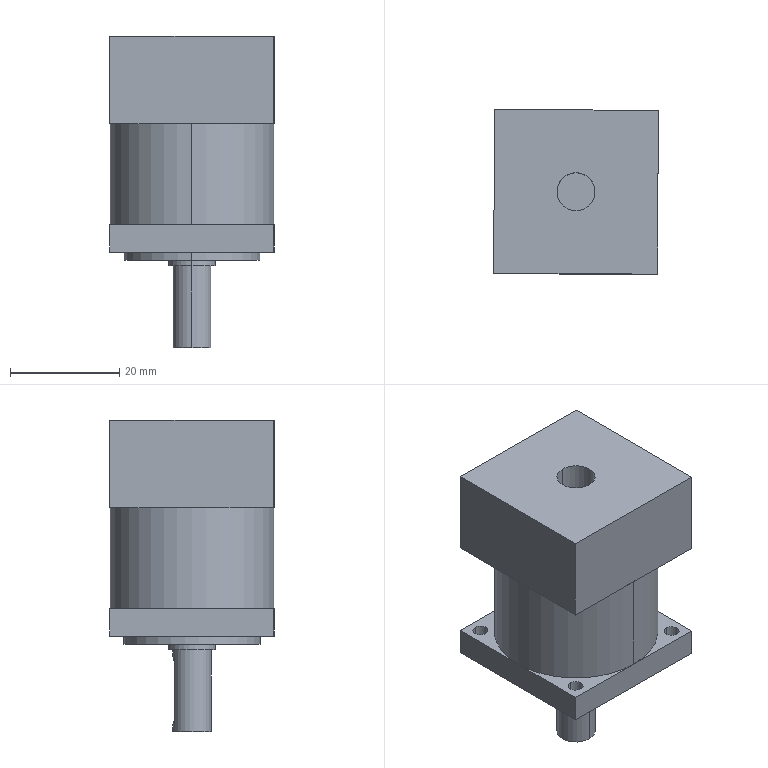Part | STEP file | 2026.6.15-Main Assembly图.sldasm-Part-157 | 1 solid | 47 faces | box 30.153 x 30.153 x 57 mm | volume 32608 mm3 | plane 25 | cylinder 22 | commonest cylinder face diameters 2.75 x8 2.5 x4 7 x4 8.5 x2 25 x2 30 x2
STEP:
#1=CARTESIAN_POINT('',(-1556.397,1436.505,3721.32));
#2=VERTEX_POINT('',#1);
#3=CARTESIAN_POINT('',(-1555.189,1436.504,3720.071));
#4=VERTEX_POINT('',#3);
#5=CARTESIAN_POINT('',(-1556.439,1436.505,3720.071));
#6=DIRECTION('',(0.0007664,1.,0.));
#7=DIRECTION('',(0.03353,-0.0000257,0.9994));
#8=AXIS2_PLACEMENT_3D('',#5,#6,#7);
#9=CIRCLE('',#8,1.25);
#10=EDGE_CURVE('',#2,#4,#9,.T.);
#11=ORIENTED_EDGE('',*,*,#10,.F.);
#12=CARTESIAN_POINT('',(-1556.396,1438.004,3721.32));
#13=VERTEX_POINT('',#12);
#14=CARTESIAN_POINT('',(-1556.395,1439.005,3721.32));
#15=DIRECTION('',(0.0007664,1.,0.));
#16=VECTOR('',#15,1000.);
#17=LINE('',#14,#16);
#18=EDGE_CURVE('',#2,#13,#17,.T.);
#19=ORIENTED_EDGE('',*,*,#18,.T.);
#20=CARTESIAN_POINT('',(-1555.188,1437.767,3720.071));
#21=VERTEX_POINT('',#20);
#22=CARTESIAN_POINT('',(-1555.188,1437.767,3720.071));
#23=CARTESIAN_POINT('',(-1555.188,1437.767,3720.234));
#24=CARTESIAN_POINT('',(-1555.22,1437.78,3720.394));
#25=CARTESIAN_POINT('',(-1555.341,1437.823,3720.691));
#26=CARTESIAN_POINT('',(-1555.43,1437.853,3720.826));
#27=CARTESIAN_POINT('',(-1555.65,1437.913,3721.054));
#28=CARTESIAN_POINT('',(-1555.783,1437.943,3721.147));
#29=CARTESIAN_POINT('',(-1556.073,1437.987,3721.277));
#30=CARTESIAN_POINT('',(-1556.234,1438.002,3721.315));
#31=CARTESIAN_POINT('',(-1556.396,1438.004,3721.32));
#32=B_SPLINE_CURVE_WITH_KNOTS('',3,(#22,#23,#24,#25,#26,#27,#28,#29,#30,#31),.UNSPECIFIED.,.F.,.F.,(4,2,2,2,4),(0.,0.0004821,0.0009642,0.001446,0.001928),.UNSPECIFIED.);
#33=EDGE_CURVE('',#21,#13,#32,.T.);
#34=ORIENTED_EDGE('',*,*,#33,.F.);
#35=CARTESIAN_POINT('',(-1555.187,1439.004,3720.071));
#36=DIRECTION('',(0.0007664,1.,0.));
#37=VECTOR('',#36,1000.);
#38=LINE('',#35,#37);
#39=EDGE_CURVE('',#4,#21,#38,.T.);
#40=ORIENTED_EDGE('',*,*,#39,.F.);
#41=EDGE_LOOP('',(#11,#19,#34,#40));
#42=FACE_OUTER_BOUND('',#41,.T.);
#43=CARTESIAN_POINT('',(-1556.437,1439.005,3720.071));
#44=DIRECTION('',(0.0007664,1.,0.));
#45=DIRECTION('',(0.03353,-0.0000257,0.9994));
#46=AXIS2_PLACEMENT_3D('',#43,#44,#45);
#47=CYLINDRICAL_SURFACE('',#46,1.25);
#48=ADVANCED_FACE('',(#42),#47,.F.);
#49=CARTESIAN_POINT('',(-1556.48,1438.005,3708.821));
#50=VERTEX_POINT('',#49);
#51=CARTESIAN_POINT('',(-1556.453,1438.005,3708.821));
#52=VERTEX_POINT('',#51);
#53=CARTESIAN_POINT('',(-1556.48,1438.005,3708.821));
#54=CARTESIAN_POINT('',(-1556.471,1438.005,3708.821));
#55=CARTESIAN_POINT('',(-1556.462,1438.005,3708.821));
#56=CARTESIAN_POINT('',(-1556.453,1438.005,3708.821));
#57=B_SPLINE_CURVE_WITH_KNOTS('',3,(#53,#54,#55,#56),.UNSPECIFIED.,.F.,.F.,(4,4),(-0.00004139,-0.00001499),.UNSPECIFIED.);
#58=EDGE_CURVE('',#50,#52,#57,.T.);
#59=ORIENTED_EDGE('',*,*,#58,.F.);
#60=CARTESIAN_POINT('',(-1556.481,1436.505,3708.821));
#61=VERTEX_POINT('',#60);
#62=CARTESIAN_POINT('',(-1556.479,1439.005,3708.821));
#63=DIRECTION('',(-0.0007664,-1.,0.));
#64=VECTOR('',#63,1000.);
#65=LINE('',#62,#64);
#66=EDGE_CURVE('',#50,#61,#65,.T.);
#67=ORIENTED_EDGE('',*,*,#66,.T.);
#68=CARTESIAN_POINT('',(-1555.189,1436.504,3710.071));
#69=VERTEX_POINT('',#68);
#70=CARTESIAN_POINT('',(-1556.439,1436.505,3710.071));
#71=DIRECTION('',(0.0007664,1.,0.));
#72=DIRECTION('',(0.03353,-0.0000257,0.9994));
#73=AXIS2_PLACEMENT_3D('',#70,#71,#72);
#74=CIRCLE('',#73,1.25);
#75=EDGE_CURVE('',#69,#61,#74,.T.);
#76=ORIENTED_EDGE('',*,*,#75,.F.);
#77=CARTESIAN_POINT('',(-1555.188,1437.767,3710.071));
#78=VERTEX_POINT('',#77);
#79=CARTESIAN_POINT('',(-1555.187,1439.004,3710.071));
#80=DIRECTION('',(-0.0007664,-1.,0.));
#81=VECTOR('',#80,1000.);
#82=LINE('',#79,#81);
#83=EDGE_CURVE('',#78,#69,#82,.T.);
#84=ORIENTED_EDGE('',*,*,#83,.F.);
#85=CARTESIAN_POINT('',(-1556.453,1438.005,3708.821));
#86=CARTESIAN_POINT('',(-1556.286,1438.005,3708.819));
#87=CARTESIAN_POINT('',(-1556.12,1437.992,3708.851));
#88=CARTESIAN_POINT('',(-1555.814,1437.949,3708.975));
#89=CARTESIAN_POINT('',(-1555.675,1437.919,3709.067));
#90=CARTESIAN_POINT('',(-1555.444,1437.857,3709.296));
#91=CARTESIAN_POINT('',(-1555.35,1437.826,3709.435));
#92=CARTESIAN_POINT('',(-1555.223,1437.781,3709.737));
#93=CARTESIAN_POINT('',(-1555.188,1437.767,3709.903));
#94=CARTESIAN_POINT('',(-1555.188,1437.767,3710.071));
#95=B_SPLINE_CURVE_WITH_KNOTS('',3,(#85,#86,#87,#88,#89,#90,#91,#92,#93,#94),.UNSPECIFIED.,.F.,.F.,(4,2,2,2,4),(-0.00001499,0.0004812,0.0009775,0.001474,0.00197),.UNSPECIFIED.);
#96=EDGE_CURVE('',#52,#78,#95,.T.);
#97=ORIENTED_EDGE('',*,*,#96,.F.);
#98=EDGE_LOOP('',(#59,#67,#76,#84,#97));
#99=FACE_OUTER_BOUND('',#98,.T.);
#100=CARTESIAN_POINT('',(-1556.437,1439.005,3710.071));
#101=DIRECTION('',(-0.0007664,-1.,0.));
#102=DIRECTION('',(-0.03353,0.0000257,-0.9994));
#103=AXIS2_PLACEMENT_3D('',#100,#101,#102);
#104=CYLINDRICAL_SURFACE('',#103,1.25);
#105=ADVANCED_FACE('',(#99),#104,.F.);
#106=CARTESIAN_POINT('',(-1556.467,1419.505,3748.571));
#107=VERTEX_POINT('',#106);
#108=CARTESIAN_POINT('',(-1541.456,1434.428,3748.571));
#109=VERTEX_POINT('',#108);
#110=CARTESIAN_POINT('',(-1556.456,1434.505,3748.571));
#111=DIRECTION('',(0.,0.,1.));
#112=DIRECTION('',(-0.0007664,-1.,0.));
#113=AXIS2_PLACEMENT_3D('',#110,#111,#112);
#114=CIRCLE('',#113,15.);
#115=EDGE_CURVE('',#107,#109,#114,.T.);
#116=ORIENTED_EDGE('',*,*,#115,.F.);
#117=CARTESIAN_POINT('',(-1556.467,1419.505,3730.071));
#118=VERTEX_POINT('',#117);
#119=CARTESIAN_POINT('',(-1556.467,1419.505,3748.571));
#120=DIRECTION('',(0.,0.,-1.));
#121=VECTOR('',#120,1000.);
#122=LINE('',#119,#121);
#123=EDGE_CURVE('',#107,#118,#122,.T.);
#124=ORIENTED_EDGE('',*,*,#123,.T.);
#125=CARTESIAN_POINT('',(-1541.456,1434.428,3730.071));
#126=VERTEX_POINT('',#125);
#127=CARTESIAN_POINT('',(-1556.456,1434.505,3730.071));
#128=DIRECTION('',(0.,0.,1.));
#129=DIRECTION('',(-0.0007664,-1.,0.));
#130=AXIS2_PLACEMENT_3D('',#127,#128,#129);
#131=CIRCLE('',#130,15.);
#132=EDGE_CURVE('',#118,#126,#131,.T.);
#133=ORIENTED_EDGE('',*,*,#132,.T.);
#134=CARTESIAN_POINT('',(-1556.379,1449.505,3730.071));
#135=VERTEX_POINT('',#134);
#136=CARTESIAN_POINT('',(-1556.456,1434.505,3730.071));
#137=DIRECTION('',(0.,0.,1.));
#138=DIRECTION('',(-0.0007664,-1.,0.));
#139=AXIS2_PLACEMENT_3D('',#136,#137,#138);
#140=CIRCLE('',#139,15.);
#141=EDGE_CURVE('',#126,#135,#140,.T.);
#142=ORIENTED_EDGE('',*,*,#141,.T.);
#143=CARTESIAN_POINT('',(-1556.444,1449.505,3730.071));
#144=VERTEX_POINT('',#143);
#145=CARTESIAN_POINT('',(-1556.456,1434.505,3730.071));
#146=DIRECTION('',(0.,0.,1.));
#147=DIRECTION('',(-0.0007664,-1.,0.));
#148=AXIS2_PLACEMENT_3D('',#145,#146,#147);
#149=CIRCLE('',#148,15.);
#150=EDGE_CURVE('',#135,#144,#149,.T.);
#151=ORIENTED_EDGE('',*,*,#150,.T.);
#152=CARTESIAN_POINT('',(-1556.444,1449.505,3748.571));
#153=VERTEX_POINT('',#152);
#154=CARTESIAN_POINT('',(-1556.444,1449.505,3748.571));
#155=DIRECTION('',(0.,0.,-1.));
#156=VECTOR('',#155,1000.);
#157=LINE('',#154,#156);
#158=EDGE_CURVE('',#153,#144,#157,.T.);
#159=ORIENTED_EDGE('',*,*,#158,.F.);
#160=CARTESIAN_POINT('',(-1556.379,1449.505,3748.571));
#161=VERTEX_POINT('',#160);
#162=CARTESIAN_POINT('',(-1556.456,1434.505,3748.571));
#163=DIRECTION('',(0.,0.,1.));
#164=DIRECTION('',(-0.0007664,-1.,0.));
#165=AXIS2_PLACEMENT_3D('',#162,#163,#164);
#166=CIRCLE('',#165,15.);
#167=EDGE_CURVE('',#161,#153,#166,.T.);
#168=ORIENTED_EDGE('',*,*,#167,.F.);
#169=CARTESIAN_POINT('',(-1556.456,1434.505,3748.571));
#170=DIRECTION('',(0.,0.,1.));
#171=DIRECTION('',(-0.0007664,-1.,0.));
#172=AXIS2_PLACEMENT_3D('',#169,#170,#171);
#173=CIRCLE('',#172,15.);
#174=EDGE_CURVE('',#109,#161,#173,.T.);
#175=ORIENTED_EDGE('',*,*,#174,.F.);
#176=EDGE_LOOP('',(#116,#124,#133,#142,#151,#159,#168,#175));
#177=FACE_OUTER_BOUND('',#176,.T.);
#178=CARTESIAN_POINT('',(-1556.456,1434.505,3748.571));
#179=DIRECTION('',(0.,0.,-1.));
#180=DIRECTION('',(0.0007664,1.,0.));
#181=AXIS2_PLACEMENT_3D('',#178,#179,#180);
#182=CYLINDRICAL_SURFACE('',#181,15.);
#183=ADVANCED_FACE('',(#177),#182,.T.);
#184=CARTESIAN_POINT('',(-1556.458,1431.005,3764.571));
#185=VERTEX_POINT('',#184);
#186=CARTESIAN_POINT('',(-1556.453,1438.005,3764.571));
#187=VERTEX_POINT('',#186);
#188=CARTESIAN_POINT('',(-1556.456,1434.505,3764.571));
#189=DIRECTION('',(0.,0.,-1.));
#190=DIRECTION('',(0.0007664,1.,0.));
#191=AXIS2_PLACEMENT_3D('',#188,#189,#190);
#192=CIRCLE('',#191,3.5);
#193=EDGE_CURVE('',#185,#187,#192,.T.);
#194=ORIENTED_EDGE('',*,*,#193,.F.);
#195=CARTESIAN_POINT('',(-1556.458,1431.005,3749.571));
#196=VERTEX_POINT('',#195);
#197=CARTESIAN_POINT('',(-1556.458,1431.005,3764.571));
#198=DIRECTION('',(0.,0.,-1.));
#199=VECTOR('',#198,1000.);
#200=LINE('',#197,#199);
#201=EDGE_CURVE('',#185,#196,#200,.T.);
#202=ORIENTED_EDGE('',*,*,#201,.T.);
#203=CARTESIAN_POINT('',(-1556.453,1438.005,3749.571));
#204=VERTEX_POINT('',#203);
#205=CARTESIAN_POINT('',(-1556.456,1434.505,3749.571));
#206=DIRECTION('',(0.,0.,1.));
#207=DIRECTION('',(0.0007664,1.,0.));
#208=AXIS2_PLACEMENT_3D('',#205,#206,#207);
#209=CIRCLE('',#208,3.5);
#210=EDGE_CURVE('',#204,#196,#209,.T.);
#211=ORIENTED_EDGE('',*,*,#210,.F.);
#212=CARTESIAN_POINT('',(-1556.453,1438.005,3764.571));
#213=DIRECTION('',(0.,0.,-1.));
#214=VECTOR('',#213,1000.);
#215=LINE('',#212,#214);
#216=EDGE_CURVE('',#187,#204,#215,.T.);
#217=ORIENTED_EDGE('',*,*,#216,.F.);
#218=EDGE_LOOP('',(#194,#202,#211,#217));
#219=FACE_OUTER_BOUND('',#218,.T.);
#220=CARTESIAN_POINT('',(-1556.456,1434.505,3764.571));
#221=DIRECTION('',(0.,0.,-1.));
#222=DIRECTION('',(0.0007664,1.,0.));
#223=AXIS2_PLACEMENT_3D('',#220,#221,#222);
#224=CYLINDRICAL_SURFACE('',#223,3.5);
#225=ADVANCED_FACE('',(#219),#224,.F.);
#226=CARTESIAN_POINT('',(-1544.146,1420.692,3730.071));
#227=VERTEX_POINT('',#226);
#228=CARTESIAN_POINT('',(-1544.144,1423.442,3730.071));
#229=VERTEX_POINT('',#228);
#230=CARTESIAN_POINT('',(-1544.145,1422.067,3730.071));
#231=DIRECTION('',(0.,0.,-1.));
#232=DIRECTION('',(-1.,0.005111,0.));
#233=AXIS2_PLACEMENT_3D('',#230,#231,#232);
#234=CIRCLE('',#233,1.375);
#235=EDGE_CURVE('',#227,#229,#234,.T.);
#236=ORIENTED_EDGE('',*,*,#235,.F.);
#237=CARTESIAN_POINT('',(-1544.146,1420.692,3725.071));
#238=VERTEX_POINT('',#237);
#239=CARTESIAN_POINT('',(-1544.146,1420.692,3730.071));
#240=DIRECTION('',(0.,0.,-1.));
#241=VECTOR('',#240,1000.);
#242=LINE('',#239,#241);
#243=EDGE_CURVE('',#227,#238,#242,.T.);
#244=ORIENTED_EDGE('',*,*,#243,.T.);
#245=CARTESIAN_POINT('',(-1544.144,1423.442,3725.071));
#246=VERTEX_POINT('',#245);
#247=CARTESIAN_POINT('',(-1544.145,1422.067,3725.071));
#248=DIRECTION('',(0.,0.,-1.));
#249=DIRECTION('',(-1.,0.005111,0.));
#250=AXIS2_PLACEMENT_3D('',#247,#248,#249);
#251=CIRCLE('',#250,1.375);
#252=EDGE_CURVE('',#238,#246,#251,.T.);
#253=ORIENTED_EDGE('',*,*,#252,.T.);
#254=CARTESIAN_POINT('',(-1544.144,1423.442,3730.071));
#255=DIRECTION('',(0.,0.,-1.));
#256=VECTOR('',#255,1000.);
#257=LINE('',#254,#256);
#258=EDGE_CURVE('',#229,#246,#257,.T.);
#259=ORIENTED_EDGE('',*,*,#258,.F.);
#260=EDGE_LOOP('',(#236,#244,#253,#259));
#261=FACE_OUTER_BOUND('',#260,.T.);
#262=CARTESIAN_POINT('',(-1544.145,1422.067,3730.071));
#263=DIRECTION('',(0.,0.,-1.));
#264=DIRECTION('',(0.0007664,1.,0.));
#265=AXIS2_PLACEMENT_3D('',#262,#263,#264);
#266=CYLINDRICAL_SURFACE('',#265,1.375);
#267=ADVANCED_FACE('',(#261),#266,.F.);
#268=CARTESIAN_POINT('',(-1568.894,1420.819,3730.071));
#269=VERTEX_POINT('',#268);
#270=CARTESIAN_POINT('',(-1568.892,1423.569,3730.071));
#271=VERTEX_POINT('',#270);
#272=CARTESIAN_POINT('',(-1568.893,1422.194,3730.071));
#273=DIRECTION('',(0.,0.,-1.));
#274=DIRECTION('',(-1.,0.005111,0.));
#275=AXIS2_PLACEMENT_3D('',#272,#273,#274);
#276=CIRCLE('',#275,1.375);
#277=EDGE_CURVE('',#269,#271,#276,.T.);
#278=ORIENTED_EDGE('',*,*,#277,.F.);
#279=CARTESIAN_POINT('',(-1568.894,1420.819,3725.071));
#280=VERTEX_POINT('',#279);
#281=CARTESIAN_POINT('',(-1568.894,1420.819,3730.071));
#282=DIRECTION('',(0.,0.,-1.));
#283=VECTOR('',#282,1000.);
#284=LINE('',#281,#283);
#285=EDGE_CURVE('',#269,#280,#284,.T.);
#286=ORIENTED_EDGE('',*,*,#285,.T.);
#287=CARTESIAN_POINT('',(-1568.892,1423.569,3725.071));
#288=VERTEX_POINT('',#287);
#289=CARTESIAN_POINT('',(-1568.893,1422.194,3725.071));
#290=DIRECTION('',(0.,0.,-1.));
#291=DIRECTION('',(-1.,0.005111,0.));
#292=AXIS2_PLACEMENT_3D('',#289,#290,#291);
#293=CIRCLE('',#292,1.375);
#294=EDGE_CURVE('',#280,#288,#293,.T.);
#295=ORIENTED_EDGE('',*,*,#294,.T.);
#296=CARTESIAN_POINT('',(-1568.892,1423.569,3730.071));
#297=DIRECTION('',(0.,0.,-1.));
#298=VECTOR('',#297,1000.);
#299=LINE('',#296,#298);
#300=EDGE_CURVE('',#271,#288,#299,.T.);
#301=ORIENTED_EDGE('',*,*,#300,.F.);
#302=EDGE_LOOP('',(#278,#286,#295,#301));
#303=FACE_OUTER_BOUND('',#302,.T.);
#304=CARTESIAN_POINT('',(-1568.893,1422.194,3730.071));
#305=DIRECTION('',(0.,0.,-1.));
#306=DIRECTION('',(0.0007664,1.,0.));
#307=AXIS2_PLACEMENT_3D('',#304,#305,#306);
#308=CYLINDRICAL_SURFACE('',#307,1.375);
#309=ADVANCED_FACE('',(#303),#308,.F.);
#310=CARTESIAN_POINT('',(-1568.768,1445.567,3730.071));
#311=VERTEX_POINT('',#310);
#312=CARTESIAN_POINT('',(-1568.766,1448.317,3730.071));
#313=VERTEX_POINT('',#312);
#314=CARTESIAN_POINT('',(-1568.767,1446.942,3730.071));
#315=DIRECTION('',(0.,0.,-1.));
#316=DIRECTION('',(-1.,0.005111,0.));
#317=AXIS2_PLACEMENT_3D('',#314,#315,#316);
#318=CIRCLE('',#317,1.375);
#319=EDGE_CURVE('',#311,#313,#318,.T.);
#320=ORIENTED_EDGE('',*,*,#319,.F.);
#321=CARTESIAN_POINT('',(-1568.768,1445.567,3725.071));
#322=VERTEX_POINT('',#321);
#323=CARTESIAN_POINT('',(-1568.768,1445.567,3730.071));
#324=DIRECTION('',(0.,0.,-1.));
#325=VECTOR('',#324,1000.);
#326=LINE('',#323,#325);
#327=EDGE_CURVE('',#311,#322,#326,.T.);
#328=ORIENTED_EDGE('',*,*,#327,.T.);
#329=CARTESIAN_POINT('',(-1568.766,1448.317,3725.071));
#330=VERTEX_POINT('',#329);
#331=CARTESIAN_POINT('',(-1568.767,1446.942,3725.071));
#332=DIRECTION('',(0.,0.,-1.));
#333=DIRECTION('',(-1.,0.005111,0.));
#334=AXIS2_PLACEMENT_3D('',#331,#332,#333);
#335=CIRCLE('',#334,1.375);
#336=EDGE_CURVE('',#322,#330,#335,.T.);
#337=ORIENTED_EDGE('',*,*,#336,.T.);
#338=CARTESIAN_POINT('',(-1568.766,1448.317,3730.071));
#339=DIRECTION('',(0.,0.,-1.));
#340=VECTOR('',#339,1000.);
#341=LINE('',#338,#340);
#342=EDGE_CURVE('',#313,#330,#341,.T.);
#343=ORIENTED_EDGE('',*,*,#342,.F.);
#344=EDGE_LOOP('',(#320,#328,#337,#343));
#345=FACE_OUTER_BOUND('',#344,.T.);
#346=CARTESIAN_POINT('',(-1568.767,1446.942,3730.071));
#347=DIRECTION('',(0.,0.,-1.));
#348=DIRECTION('',(0.0007664,1.,0.));
#349=AXIS2_PLACEMENT_3D('',#346,#347,#348);
#350=CYLINDRICAL_SURFACE('',#349,1.375);
#351=ADVANCED_FACE('',(#345),#350,.F.);
#352=CARTESIAN_POINT('',(-1544.019,1445.441,3730.071));
#353=VERTEX_POINT('',#352);
#354=CARTESIAN_POINT('',(-1544.017,1448.191,3730.071));
#355=VERTEX_POINT('',#354);
#356=CARTESIAN_POINT('',(-1544.018,1446.816,3730.071));
#357=DIRECTION('',(0.,0.,-1.));
#358=DIRECTION('',(-1.,0.005111,0.));
#359=AXIS2_PLACEMENT_3D('',#356,#357,#358);
#360=CIRCLE('',#359,1.375);
#361=EDGE_CURVE('',#353,#355,#360,.T.);
#362=ORIENTED_EDGE('',*,*,#361,.F.);
#363=CARTESIAN_POINT('',(-1544.019,1445.441,3725.071));
#364=VERTEX_POINT('',#363);
#365=CARTESIAN_POINT('',(-1544.019,1445.441,3730.071));
#366=DIRECTION('',(0.,0.,-1.));
#367=VECTOR('',#366,1000.);
#368=LINE('',#365,#367);
#369=EDGE_CURVE('',#353,#364,#368,.T.);
#370=ORIENTED_EDGE('',*,*,#369,.T.);
#371=CARTESIAN_POINT('',(-1544.017,1448.191,3725.071));
#372=VERTEX_POINT('',#371);
#373=CARTESIAN_POINT('',(-1544.018,1446.816,3725.071));
#374=DIRECTION('',(0.,0.,-1.));
#375=DIRECTION('',(-1.,0.005111,0.));
#376=AXIS2_PLACEMENT_3D('',#373,#374,#375);
#377=CIRCLE('',#376,1.375);
#378=EDGE_CURVE('',#364,#372,#377,.T.);
#379=ORIENTED_EDGE('',*,*,#378,.T.);
#380=CARTESIAN_POINT('',(-1544.017,1448.191,3730.071));
#381=DIRECTION('',(0.,0.,-1.));
#382=VECTOR('',#381,1000.);
#383=LINE('',#380,#382);
#384=EDGE_CURVE('',#355,#372,#383,.T.);
#385=ORIENTED_EDGE('',*,*,#384,.F.);
#386=EDGE_LOOP('',(#362,#370,#379,#385));
#387=FACE_OUTER_BOUND('',#386,.T.);
#388=CARTESIAN_POINT('',(-1544.018,1446.816,3730.071));
#389=DIRECTION('',(0.,0.,-1.));
#390=DIRECTION('',(0.0007664,1.,0.));
#391=AXIS2_PLACEMENT_3D('',#388,#389,#390);
#392=CYLINDRICAL_SURFACE('',#391,1.375);
#393=ADVANCED_FACE('',(#387),#392,.F.);
#394=CARTESIAN_POINT('',(-1556.446,1447.005,3725.071));
#395=VERTEX_POINT('',#394);
#396=CARTESIAN_POINT('',(-1556.465,1422.005,3725.071));
#397=VERTEX_POINT('',#396);
#398=CARTESIAN_POINT('',(-1556.456,1434.505,3725.071));
#399=DIRECTION('',(0.,0.,-1.));
#400=DIRECTION('',(1.,-0.005111,0.));
#401=AXIS2_PLACEMENT_3D('',#398,#399,#400);
#402=CIRCLE('',#401,12.5);
#403=EDGE_CURVE('',#395,#397,#402,.T.);
#404=ORIENTED_EDGE('',*,*,#403,.T.);
#405=CARTESIAN_POINT('',(-1556.465,1422.005,3723.571));
#406=VERTEX_POINT('',#405);
#407=CARTESIAN_POINT('',(-1556.465,1422.005,3725.071));
#408=DIRECTION('',(0.,0.,-1.));
#409=VECTOR('',#408,1000.);
#410=LINE('',#407,#409);
#411=EDGE_CURVE('',#397,#406,#410,.T.);
#412=ORIENTED_EDGE('',*,*,#411,.T.);
#413=CARTESIAN_POINT('',(-1556.446,1447.005,3723.571));
#414=VERTEX_POINT('',#413);
#415=CARTESIAN_POINT('',(-1556.456,1434.505,3723.571));
#416=DIRECTION('',(0.,0.,-1.));
#417=DIRECTION('',(1.,-0.005111,0.));
#418=AXIS2_PLACEMENT_3D('',#415,#416,#417);
#419=CIRCLE('',#418,12.5);
#420=EDGE_CURVE('',#414,#406,#419,.T.);
#421=ORIENTED_EDGE('',*,*,#420,.F.);
#422=CARTESIAN_POINT('',(-1556.446,1447.005,3725.071));
#423=DIRECTION('',(0.,0.,-1.));
#424=VECTOR('',#423,1000.);
#425=LINE('',#422,#424);
#426=EDGE_CURVE('',#395,#414,#425,.T.);
#427=ORIENTED_EDGE('',*,*,#426,.F.);
#428=EDGE_LOOP('',(#404,#412,#421,#427));
#429=FACE_OUTER_BOUND('',#428,.T.);
#430=CARTESIAN_POINT('',(-1556.456,1434.505,3725.071));
#431=DIRECTION('',(0.,0.,-1.));
#432=DIRECTION('',(0.0007664,1.,0.));
#433=AXIS2_PLACEMENT_3D('',#430,#431,#432);
#434=CYLINDRICAL_SURFACE('',#433,12.5);
#435=ADVANCED_FACE('',(#429),#434,.T.);
#436=CARTESIAN_POINT('',(-1556.453,1438.755,3723.571));
#437=VERTEX_POINT('',#436);
#438=CARTESIAN_POINT('',(-1556.459,1430.255,3723.571));
#439=VERTEX_POINT('',#438);
#440=CARTESIAN_POINT('',(-1556.456,1434.505,3723.571));
#441=DIRECTION('',(0.,0.,-1.));
#442=DIRECTION('',(-1.,0.005111,0.));
#443=AXIS2_PLACEMENT_3D('',#440,#441,#442);
#444=CIRCLE('',#443,4.25);
#445=EDGE_CURVE('',#437,#439,#444,.T.);
#446=ORIENTED_EDGE('',*,*,#445,.T.);
#447=CARTESIAN_POINT('',(-1556.459,1430.255,3722.571));
#448=VERTEX_POINT('',#447);
#449=CARTESIAN_POINT('',(-1556.459,1430.255,3723.571));
#450=DIRECTION('',(0.,0.,-1.));
#451=VECTOR('',#450,1000.);
#452=LINE('',#449,#451);
#453=EDGE_CURVE('',#439,#448,#452,.T.);
#454=ORIENTED_EDGE('',*,*,#453,.T.);
#455=CARTESIAN_POINT('',(-1556.453,1438.755,3722.571));
#456=VERTEX_POINT('',#455);
#457=CARTESIAN_POINT('',(-1556.456,1434.505,3722.571));
#458=DIRECTION('',(0.,0.,-1.));
#459=DIRECTION('',(-1.,0.005111,0.));
#460=AXIS2_PLACEMENT_3D('',#457,#458,#459);
#461=CIRCLE('',#460,4.25);
#462=EDGE_CURVE('',#456,#448,#461,.T.);
#463=ORIENTED_EDGE('',*,*,#462,.F.);
#464=CARTESIAN_POINT('',(-1556.453,1438.755,3723.571));
#465=DIRECTION('',(0.,0.,-1.));
#466=VECTOR('',#465,1000.);
#467=LINE('',#464,#466);
#468=EDGE_CURVE('',#437,#456,#467,.T.);
#469=ORIENTED_EDGE('',*,*,#468,.F.);
#470=EDGE_LOOP('',(#446,#454,#463,#469));
#471=FACE_OUTER_BOUND('',#470,.T.);
#472=CARTESIAN_POINT('',(-1556.456,1434.505,3723.571));
#473=DIRECTION('',(0.,0.,-1.));
#474=DIRECTION('',(0.0007664,1.,0.));
#475=AXIS2_PLACEMENT_3D('',#472,#473,#474);
#476=CYLINDRICAL_SURFACE('',#475,4.25);
#477=ADVANCED_FACE('',(#471),#476,.T.);
#478=CARTESIAN_POINT('',(-1556.453,1438.005,3722.571));
#479=VERTEX_POINT('',#478);
#480=CARTESIAN_POINT('',(-1556.458,1431.005,3722.571));
#481=VERTEX_POINT('',#480);
#482=CARTESIAN_POINT('',(-1556.456,1434.505,3722.571));
#483=DIRECTION('',(0.,0.,-1.));
#484=DIRECTION('',(-1.,0.005111,0.));
#485=AXIS2_PLACEMENT_3D('',#482,#483,#484);
#486=CIRCLE('',#485,3.5);
#487=EDGE_CURVE('',#479,#481,#486,.T.);
#488=ORIENTED_EDGE('',*,*,#487,.T.);
#489=CARTESIAN_POINT('',(-1556.458,1431.005,3707.571));
#490=VERTEX_POINT('',#489);
#491=CARTESIAN_POINT('',(-1556.458,1431.005,3722.571));
#492=DIRECTION('',(0.,0.,-1.));
#493=VECTOR('',#492,1000.);
#494=LINE('',#491,#493);
#495=EDGE_CURVE('',#481,#490,#494,.T.);
#496=ORIENTED_EDGE('',*,*,#495,.T.);
#497=CARTESIAN_POINT('',(-1556.453,1438.005,3707.571));
#498=VERTEX_POINT('',#497);
#499=CARTESIAN_POINT('',(-1556.456,1434.505,3707.571));
#500=DIRECTION('',(0.,0.,-1.));
#501=DIRECTION('',(-1.,0.005111,0.));
#502=AXIS2_PLACEMENT_3D('',#499,#500,#501);
#503=CIRCLE('',#502,3.5);
#504=EDGE_CURVE('',#498,#490,#503,.T.);
#505=ORIENTED_EDGE('',*,*,#504,.F.);
#506=CARTESIAN_POINT('',(-1556.453,1438.005,3722.571));
#507=DIRECTION('',(0.,0.,-1.));
#508=VECTOR('',#507,1000.);
#509=LINE('',#506,#508);
#510=EDGE_CURVE('',#52,#498,#509,.T.);
#511=ORIENTED_EDGE('',*,*,#510,.F.);
#512=ORIENTED_EDGE('',*,*,#96,.T.);
#513=CARTESIAN_POINT('',(-1555.188,1437.767,3722.571));
#514=DIRECTION('',(0.,0.,1.));
#515=VECTOR('',#514,1000.);
#516=LINE('',#513,#515);
#517=EDGE_CURVE('',#78,#21,#516,.T.);
#518=ORIENTED_EDGE('',*,*,#517,.T.);
#519=ORIENTED_EDGE('',*,*,#33,.T.);
#520=CARTESIAN_POINT('',(-1556.453,1438.005,3721.321));
#521=VERTEX_POINT('',#520);
#522=CARTESIAN_POINT('',(-1556.396,1438.004,3721.32));
#523=CARTESIAN_POINT('',(-1556.415,1438.005,3721.321));
#524=CARTESIAN_POINT('',(-1556.434,1438.005,3721.321));
#525=CARTESIAN_POINT('',(-1556.453,1438.005,3721.321));
#526=B_SPLINE_CURVE_WITH_KNOTS('',3,(#522,#523,#524,#525),.UNSPECIFIED.,.F.,.F.,(4,4),(0.001928,0.001985),.UNSPECIFIED.);
#527=EDGE_CURVE('',#13,#521,#526,.T.);
#528=ORIENTED_EDGE('',*,*,#527,.T.);
#529=CARTESIAN_POINT('',(-1556.453,1438.005,3722.571));
#530=DIRECTION('',(0.,0.,-1.));
#531=VECTOR('',#530,1000.);
#532=LINE('',#529,#531);
#533=EDGE_CURVE('',#479,#521,#532,.T.);
#534=ORIENTED_EDGE('',*,*,#533,.F.);
#535=EDGE_LOOP('',(#488,#496,#505,#511,#512,#518,#519,#528,#534));
#536=FACE_OUTER_BOUND('',#535,.T.);
#537=CARTESIAN_POINT('',(-1556.456,1434.505,3722.571));
#538=DIRECTION('',(0.,0.,-1.));
#539=DIRECTION('',(0.0007664,1.,0.));
#540=AXIS2_PLACEMENT_3D('',#537,#538,#539);
#541=CYLINDRICAL_SURFACE('',#540,3.5);
#542=ADVANCED_FACE('',(#536),#541,.T.);
#543=ORIENTED_EDGE('',*,*,#495,.F.);
#544=CARTESIAN_POINT('',(-1556.456,1434.505,3722.571));
#545=DIRECTION('',(0.,0.,-1.));
#546=DIRECTION('',(-1.,0.005111,0.));
#547=AXIS2_PLACEMENT_3D('',#544,#545,#546);
#548=CIRCLE('',#547,3.5);
#549=EDGE_CURVE('',#481,#479,#548,.T.);
#550=ORIENTED_EDGE('',*,*,#549,.T.);
#551=ORIENTED_EDGE('',*,*,#533,.T.);
#552=CARTESIAN_POINT('',(-1557.688,1437.781,3720.071));
#553=VERTEX_POINT('',#552);
#554=CARTESIAN_POINT('',(-1556.453,1438.005,3721.321));
#555=CARTESIAN_POINT('',(-1556.618,1438.005,3721.319));
#556=CARTESIAN_POINT('',(-1556.78,1437.993,3721.284));
#557=CARTESIAN_POINT('',(-1557.078,1437.952,3721.156));
#558=CARTESIAN_POINT('',(-1557.214,1437.924,3721.063));
#559=CARTESIAN_POINT('',(-1557.44,1437.866,3720.835));
#560=CARTESIAN_POINT('',(-1557.531,1437.836,3720.698));
#561=CARTESIAN_POINT('',(-1557.655,1437.794,3720.4));
#562=CARTESIAN_POINT('',(-1557.688,1437.781,3720.236));
#563=CARTESIAN_POINT('',(-1557.688,1437.781,3720.071));
#564=B_SPLINE_CURVE_WITH_KNOTS('',3,(#554,#555,#556,#557,#558,#559,#560,#561,#562,#563),.UNSPECIFIED.,.F.,.F.,(4,2,2,2,4),(0.001985,0.002473,0.002962,0.00345,0.003938),.UNSPECIFIED.);
#565=EDGE_CURVE('',#521,#553,#564,.T.);
#566=ORIENTED_EDGE('',*,*,#565,.T.);
#567=CARTESIAN_POINT('',(-1557.688,1437.781,3710.071));
#568=VERTEX_POINT('',#567);
#569=CARTESIAN_POINT('',(-1557.688,1437.781,3722.571));
#570=DIRECTION('',(0.,0.,1.));
#571=VECTOR('',#570,1000.);
#572=LINE('',#569,#571);
#573=EDGE_CURVE('',#568,#553,#572,.T.);
#574=ORIENTED_EDGE('',*,*,#573,.F.);
#575=CARTESIAN_POINT('',(-1557.688,1437.781,3710.071));
#576=CARTESIAN_POINT('',(-1557.688,1437.781,3709.908));
#577=CARTESIAN_POINT('',(-1557.656,1437.793,3709.748));
#578=CARTESIAN_POINT('',(-1557.535,1437.835,3709.451));
#579=CARTESIAN_POINT('',(-1557.447,1437.864,3709.316));
#580=CARTESIAN_POINT('',(-1557.227,1437.921,3709.088));
#581=CARTESIAN_POINT('',(-1557.093,1437.949,3708.994));
#582=CARTESIAN_POINT('',(-1556.803,1437.991,3708.865));
#583=CARTESIAN_POINT('',(-1556.642,1438.004,3708.827));
#584=CARTESIAN_POINT('',(-1556.48,1438.005,3708.821));
#585=B_SPLINE_CURVE_WITH_KNOTS('',3,(#575,#576,#577,#578,#579,#580,#581,#582,#583,#584),.UNSPECIFIED.,.F.,.F.,(4,2,2,2,4),(-0.001969,-0.001487,-0.001005,-0.0005232,-0.00004139),.UNSPECIFIED.);
#586=EDGE_CURVE('',#568,#50,#585,.T.);
#587=ORIENTED_EDGE('',*,*,#586,.T.);
#588=ORIENTED_EDGE('',*,*,#58,.T.);
#589=ORIENTED_EDGE('',*,*,#510,.T.);
#590=CARTESIAN_POINT('',(-1556.456,1434.505,3707.571));
#591=DIRECTION('',(0.,0.,-1.));
#592=DIRECTION('',(-1.,0.005111,0.));
#593=AXIS2_PLACEMENT_3D('',#590,#591,#592);
#594=CIRCLE('',#593,3.5);
#595=EDGE_CURVE('',#490,#498,#594,.T.);
#596=ORIENTED_EDGE('',*,*,#595,.F.);
#597=EDGE_LOOP('',(#543,#550,#551,#566,#574,#587,#588,#589,#596));
#598=FACE_OUTER_BOUND('',#597,.T.);
#599=CARTESIAN_POINT('',(-1556.456,1434.505,3722.571));
#600=DIRECTION('',(0.,0.,-1.));
#601=DIRECTION('',(0.0007664,1.,0.));
#602=AXIS2_PLACEMENT_3D('',#599,#600,#601);
#603=CYLINDRICAL_SURFACE('',#602,3.5);
#604=ADVANCED_FACE('',(#598),#603,.T.);
#605=ORIENTED_EDGE('',*,*,#504,.T.);
#606=ORIENTED_EDGE('',*,*,#595,.T.);
#607=EDGE_LOOP('',(#605,#606));
#608=FACE_OUTER_BOUND('',#607,.T.);
#609=CARTESIAN_POINT('',(-1556.456,1434.505,3707.571));
#610=DIRECTION('',(0.,0.,-1.));
#611=DIRECTION('',(0.0007664,1.,0.));
#612=AXIS2_PLACEMENT_3D('',#609,#610,#611);
#613=PLANE('',#612);
#614=ADVANCED_FACE('',(#608),#613,.T.);
#615=ORIENTED_EDGE('',*,*,#453,.F.);
#616=CARTESIAN_POINT('',(-1556.456,1434.505,3723.571));
#617=DIRECTION('',(0.,0.,-1.));
#618=DIRECTION('',(-1.,0.005111,0.));
#619=AXIS2_PLACEMENT_3D('',#616,#617,#618);
#620=CIRCLE('',#619,4.25);
#621=EDGE_CURVE('',#439,#437,#620,.T.);
#622=ORIENTED_EDGE('',*,*,#621,.T.);
#623=ORIENTED_EDGE('',*,*,#468,.T.);
#624=CARTESIAN_POINT('',(-1556.456,1434.505,3722.571));
#625=DIRECTION('',(0.,0.,-1.));
#626=DIRECTION('',(-1.,0.005111,0.));
#627=AXIS2_PLACEMENT_3D('',#624,#625,#626);
#628=CIRCLE('',#627,4.25);
#629=EDGE_CURVE('',#448,#456,#628,.T.);
#630=ORIENTED_EDGE('',*,*,#629,.F.);
#631=EDGE_LOOP('',(#615,#622,#623,#630));
#632=FACE_OUTER_BOUND('',#631,.T.);
#633=CARTESIAN_POINT('',(-1556.456,1434.505,3723.571));
#634=DIRECTION('',(0.,0.,-1.));
#635=DIRECTION('',(0.0007664,1.,0.));
#636=AXIS2_PLACEMENT_3D('',#633,#634,#635);
#637=CYLINDRICAL_SURFACE('',#636,4.25);
#638=ADVANCED_FACE('',(#632),#637,.T.);
#639=ORIENTED_EDGE('',*,*,#487,.F.);
#640=ORIENTED_EDGE('',*,*,#549,.F.);
#641=EDGE_LOOP('',(#639,#640));
#642=FACE_BOUND('',#641,.T.);
#643=ORIENTED_EDGE('',*,*,#462,.T.);
#644=ORIENTED_EDGE('',*,*,#629,.T.);
#645=EDGE_LOOP('',(#643,#644));
#646=FACE_OUTER_BOUND('',#645,.T.);
#647=CARTESIAN_POINT('',(-1556.456,1434.505,3722.571));
#648=DIRECTION('',(0.,0.,1.));
#649=DIRECTION('',(-0.0007664,-1.,0.));
#650=AXIS2_PLACEMENT_3D('',#647,#648,#649);
#651=PLANE('',#650);
#652=ADVANCED_FACE('',(#642,#646),#651,.F.);
#653=ORIENTED_EDGE('',*,*,#411,.F.);
#654=CARTESIAN_POINT('',(-1556.456,1434.505,3725.071));
#655=DIRECTION('',(0.,0.,-1.));
#656=DIRECTION('',(1.,-0.005111,0.));
#657=AXIS2_PLACEMENT_3D('',#654,#655,#656);
#658=CIRCLE('',#657,12.5);
#659=EDGE_CURVE('',#397,#395,#658,.T.);
#660=ORIENTED_EDGE('',*,*,#659,.T.);
#661=ORIENTED_EDGE('',*,*,#426,.T.);
#662=CARTESIAN_POINT('',(-1556.456,1434.505,3723.571));
#663=DIRECTION('',(0.,0.,-1.));
#664=DIRECTION('',(1.,-0.005111,0.));
#665=AXIS2_PLACEMENT_3D('',#662,#663,#664);
#666=CIRCLE('',#665,12.5);
#667=EDGE_CURVE('',#406,#414,#666,.T.);
#668=ORIENTED_EDGE('',*,*,#667,.F.);
#669=EDGE_LOOP('',(#653,#660,#661,#668));
#670=FACE_OUTER_BOUND('',#669,.T.);
#671=CARTESIAN_POINT('',(-1556.456,1434.505,3725.071));
#672=DIRECTION('',(0.,0.,-1.));
#673=DIRECTION('',(0.0007664,1.,0.));
#674=AXIS2_PLACEMENT_3D('',#671,#672,#673);
#675=CYLINDRICAL_SURFACE('',#674,12.5);
#676=ADVANCED_FACE('',(#670),#675,.T.);
#677=ORIENTED_EDGE('',*,*,#445,.F.);
#678=ORIENTED_EDGE('',*,*,#621,.F.);
#679=EDGE_LOOP('',(#677,#678));
#680=FACE_BOUND('',#679,.T.);
#681=ORIENTED_EDGE('',*,*,#420,.T.);
#682=ORIENTED_EDGE('',*,*,#667,.T.);
#683=EDGE_LOOP('',(#681,#682));
#684=FACE_OUTER_BOUND('',#683,.T.);
#685=CARTESIAN_POINT('',(-1556.456,1434.505,3723.571));
#686=DIRECTION('',(0.,0.,-1.));
#687=DIRECTION('',(0.0007664,1.,0.));
#688=AXIS2_PLACEMENT_3D('',#685,#686,#687);
#689=PLANE('',#688);
#690=ADVANCED_FACE('',(#680,#684),#689,.T.);
#691=ORIENTED_EDGE('',*,*,#141,.F.);
#692=CARTESIAN_POINT('',(-1541.379,1449.428,3730.071));
#693=VERTEX_POINT('',#692);
#694=CARTESIAN_POINT('',(-1541.379,1449.428,3730.071));
#695=DIRECTION('',(-0.005111,-1.,0.));
#696=VECTOR('',#695,1000.);
#697=LINE('',#694,#696);
#698=EDGE_CURVE('',#693,#126,#697,.T.);
#699=ORIENTED_EDGE('',*,*,#698,.F.);
#700=CARTESIAN_POINT('',(-1571.379,1449.581,3730.071));
#701=DIRECTION('',(1.,-0.005111,0.));
#702=VECTOR('',#701,1000.);
#703=LINE('',#700,#702);
#704=EDGE_CURVE('',#135,#693,#703,.T.);
#705=ORIENTED_EDGE('',*,*,#704,.F.);
#706=EDGE_LOOP('',(#691,#699,#705));
#707=FACE_OUTER_BOUND('',#706,.T.);
#708=CARTESIAN_POINT('',(-1544.018,1446.816,3730.071));
#709=DIRECTION('',(0.,0.,-1.));
#710=DIRECTION('',(-1.,0.005111,0.));
#711=AXIS2_PLACEMENT_3D('',#708,#709,#710);
#712=CIRCLE('',#711,1.375);
#713=EDGE_CURVE('',#355,#353,#712,.T.);
#714=ORIENTED_EDGE('',*,*,#713,.T.);
#715=ORIENTED_EDGE('',*,*,#361,.T.);
#716=EDGE_LOOP('',(#714,#715));
#717=FACE_BOUND('',#716,.T.);
#718=CARTESIAN_POINT('',(-1568.893,1422.194,3730.071));
#719=DIRECTION('',(0.,0.,-1.));
#720=DIRECTION('',(0.0007664,1.,0.));
#721=AXIS2_PLACEMENT_3D('',#718,#719,#720);
#722=PLANE('',#721);
#723=ADVANCED_FACE('',(#707,#717),#722,.F.);
#724=ORIENTED_EDGE('',*,*,#150,.F.);
#725=CARTESIAN_POINT('',(-1571.379,1449.581,3730.071));
#726=VERTEX_POINT('',#725);
#727=CARTESIAN_POINT('',(-1571.379,1449.581,3730.071));
#728=DIRECTION('',(1.,-0.005111,0.));
#729=VECTOR('',#728,1000.);
#730=LINE('',#727,#729);
#731=EDGE_CURVE('',#726,#135,#730,.T.);
#732=ORIENTED_EDGE('',*,*,#731,.F.);
#733=CARTESIAN_POINT('',(-1571.456,1434.581,3730.071));
#734=VERTEX_POINT('',#733);
#735=CARTESIAN_POINT('',(-1571.532,1419.582,3730.071));
#736=DIRECTION('',(0.005111,1.,0.));
#737=VECTOR('',#736,1000.);
#738=LINE('',#735,#737);
#739=EDGE_CURVE('',#734,#726,#738,.T.);
#740=ORIENTED_EDGE('',*,*,#739,.F.);
#741=CARTESIAN_POINT('',(-1556.456,1434.505,3730.071));
#742=DIRECTION('',(0.,0.,1.));
#743=DIRECTION('',(-0.0007664,-1.,0.));
#744=AXIS2_PLACEMENT_3D('',#741,#742,#743);
#745=CIRCLE('',#744,15.);
#746=EDGE_CURVE('',#144,#734,#745,.T.);
#747=ORIENTED_EDGE('',*,*,#746,.F.);
#748=EDGE_LOOP('',(#724,#732,#740,#747));
#749=FACE_OUTER_BOUND('',#748,.T.);
#750=CARTESIAN_POINT('',(-1568.767,1446.942,3730.071));
#751=DIRECTION('',(0.,0.,-1.));
#752=DIRECTION('',(-1.,0.005111,0.));
#753=AXIS2_PLACEMENT_3D('',#750,#751,#752);
#754=CIRCLE('',#753,1.375);
#755=EDGE_CURVE('',#313,#311,#754,.T.);
#756=ORIENTED_EDGE('',*,*,#755,.T.);
#757=ORIENTED_EDGE('',*,*,#319,.T.);
#758=EDGE_LOOP('',(#756,#757));
#759=FACE_BOUND('',#758,.T.);
#760=CARTESIAN_POINT('',(-1568.893,1422.194,3730.071));
#761=DIRECTION('',(0.,0.,-1.));
#762=DIRECTION('',(0.0007664,1.,0.));
#763=AXIS2_PLACEMENT_3D('',#760,#761,#762);
#764=PLANE('',#763);
#765=ADVANCED_FACE('',(#749,#759),#764,.F.);
#766=CARTESIAN_POINT('',(-1556.532,1419.505,3730.071));
#767=VERTEX_POINT('',#766);
#768=CARTESIAN_POINT('',(-1556.456,1434.505,3730.071));
#769=DIRECTION('',(0.,0.,1.));
#770=DIRECTION('',(-0.0007664,-1.,0.));
#771=AXIS2_PLACEMENT_3D('',#768,#769,#770);
#772=CIRCLE('',#771,15.);
#773=EDGE_CURVE('',#734,#767,#772,.T.);
#774=ORIENTED_EDGE('',*,*,#773,.F.);
#775=CARTESIAN_POINT('',(-1571.532,1419.582,3730.071));
#776=VERTEX_POINT('',#775);
#777=CARTESIAN_POINT('',(-1571.532,1419.582,3730.071));
#778=DIRECTION('',(0.005111,1.,0.));
#779=VECTOR('',#778,1000.);
#780=LINE('',#777,#779);
#781=EDGE_CURVE('',#776,#734,#780,.T.);
#782=ORIENTED_EDGE('',*,*,#781,.F.);
#783=CARTESIAN_POINT('',(-1541.533,1419.428,3730.071));
#784=DIRECTION('',(-1.,0.005111,0.));
#785=VECTOR('',#784,1000.);
#786=LINE('',#783,#785);
#787=EDGE_CURVE('',#767,#776,#786,.T.);
#788=ORIENTED_EDGE('',*,*,#787,.F.);
#789=EDGE_LOOP('',(#774,#782,#788));
#790=FACE_OUTER_BOUND('',#789,.T.);
#791=CARTESIAN_POINT('',(-1568.893,1422.194,3730.071));
#792=DIRECTION('',(0.,0.,-1.));
#793=DIRECTION('',(-1.,0.005111,0.));
#794=AXIS2_PLACEMENT_3D('',#791,#792,#793);
#795=CIRCLE('',#794,1.375);
#796=EDGE_CURVE('',#271,#269,#795,.T.);
#797=ORIENTED_EDGE('',*,*,#796,.T.);
#798=ORIENTED_EDGE('',*,*,#277,.T.);
#799=EDGE_LOOP('',(#797,#798));
#800=FACE_BOUND('',#799,.T.);
#801=CARTESIAN_POINT('',(-1568.893,1422.194,3730.071));
#802=DIRECTION('',(0.,0.,-1.));
#803=DIRECTION('',(0.0007664,1.,0.));
#804=AXIS2_PLACEMENT_3D('',#801,#802,#803);
#805=PLANE('',#804);
#806=ADVANCED_FACE('',(#790,#800),#805,.F.);
#807=CARTESIAN_POINT('',(-1571.379,1449.581,3725.071));
#808=VERTEX_POINT('',#807);
#809=CARTESIAN_POINT('',(-1541.379,1449.428,3725.071));
#810=VERTEX_POINT('',#809);
#811=CARTESIAN_POINT('',(-1571.379,1449.581,3725.071));
#812=DIRECTION('',(1.,-0.005111,0.));
#813=VECTOR('',#812,1000.);
#814=LINE('',#811,#813);
#815=EDGE_CURVE('',#808,#810,#814,.T.);
#816=ORIENTED_EDGE('',*,*,#815,.F.);
#817=CARTESIAN_POINT('',(-1571.379,1449.581,3730.071));
#818=DIRECTION('',(0.,0.,-1.));
#819=VECTOR('',#818,1000.);
#820=LINE('',#817,#819);
#821=EDGE_CURVE('',#726,#808,#820,.T.);
#822=ORIENTED_EDGE('',*,*,#821,.F.);
#823=ORIENTED_EDGE('',*,*,#731,.T.);
#824=ORIENTED_EDGE('',*,*,#704,.T.);
#825=CARTESIAN_POINT('',(-1541.379,1449.428,3730.071));
#826=DIRECTION('',(0.,0.,-1.));
#827=VECTOR('',#826,1000.);
#828=LINE('',#825,#827);
#829=EDGE_CURVE('',#693,#810,#828,.T.);
#830=ORIENTED_EDGE('',*,*,#829,.T.);
#831=EDGE_LOOP('',(#816,#822,#823,#824,#830));
#832=FACE_OUTER_BOUND('',#831,.T.);
#833=CARTESIAN_POINT('',(-1571.379,1449.581,3730.071));
#834=DIRECTION('',(0.005111,1.,0.));
#835=DIRECTION('',(0.03353,-0.0001714,0.9994));
#836=AXIS2_PLACEMENT_3D('',#833,#834,#835);
#837=PLANE('',#836);
#838=ADVANCED_FACE('',(#832),#837,.T.);
#839=CARTESIAN_POINT('',(-1541.533,1419.428,3725.071));
#840=VERTEX_POINT('',#839);
#841=CARTESIAN_POINT('',(-1541.379,1449.428,3725.071));
#842=DIRECTION('',(-0.005111,-1.,0.));
#843=VECTOR('',#842,1000.);
#844=LINE('',#841,#843);
#845=EDGE_CURVE('',#810,#840,#844,.T.);
#846=ORIENTED_EDGE('',*,*,#845,.F.);
#847=ORIENTED_EDGE('',*,*,#829,.F.);
#848=ORIENTED_EDGE('',*,*,#698,.T.);
#849=CARTESIAN_POINT('',(-1541.533,1419.428,3730.071));
#850=VERTEX_POINT('',#849);
#851=CARTESIAN_POINT('',(-1541.379,1449.428,3730.071));
#852=DIRECTION('',(-0.005111,-1.,0.));
#853=VECTOR('',#852,1000.);
#854=LINE('',#851,#853);
#855=EDGE_CURVE('',#126,#850,#854,.T.);
#856=ORIENTED_EDGE('',*,*,#855,.T.);
#857=CARTESIAN_POINT('',(-1541.533,1419.428,3730.071));
#858=DIRECTION('',(0.,0.,-1.));
#859=VECTOR('',#858,1000.);
#860=LINE('',#857,#859);
#861=EDGE_CURVE('',#850,#840,#860,.T.);
#862=ORIENTED_EDGE('',*,*,#861,.T.);
#863=EDGE_LOOP('',(#846,#847,#848,#856,#862));
#864=FACE_OUTER_BOUND('',#863,.T.);
#865=CARTESIAN_POINT('',(-1541.379,1449.428,3730.071));
#866=DIRECTION('',(1.,-0.005111,0.));
#867=DIRECTION('',(0.0006563,0.1284,-0.9917));
#868=AXIS2_PLACEMENT_3D('',#865,#866,#867);
#869=PLANE('',#868);
#870=ADVANCED_FACE('',(#864),#869,.T.);
#871=CARTESIAN_POINT('',(-1571.532,1419.582,3725.071));
#872=VERTEX_POINT('',#871);
#873=CARTESIAN_POINT('',(-1541.533,1419.428,3725.071));
#874=DIRECTION('',(-1.,0.005111,0.));
#875=VECTOR('',#874,1000.);
#876=LINE('',#873,#875);
#877=EDGE_CURVE('',#840,#872,#876,.T.);
#878=ORIENTED_EDGE('',*,*,#877,.F.);
#879=ORIENTED_EDGE('',*,*,#861,.F.);
#880=CARTESIAN_POINT('',(-1541.533,1419.428,3730.071));
#881=DIRECTION('',(-1.,0.005111,0.));
#882=VECTOR('',#881,1000.);
#883=LINE('',#880,#882);
#884=EDGE_CURVE('',#850,#767,#883,.T.);
#885=ORIENTED_EDGE('',*,*,#884,.T.);
#886=ORIENTED_EDGE('',*,*,#787,.T.);
#887=CARTESIAN_POINT('',(-1571.532,1419.582,3730.071));
#888=DIRECTION('',(0.,0.,-1.));
#889=VECTOR('',#888,1000.);
#890=LINE('',#887,#889);
#891=EDGE_CURVE('',#776,#872,#890,.T.);
#892=ORIENTED_EDGE('',*,*,#891,.T.);
#893=EDGE_LOOP('',(#878,#879,#885,#886,#892));
#894=FACE_OUTER_BOUND('',#893,.T.);
#895=CARTESIAN_POINT('',(-1541.533,1419.428,3730.071));
#896=DIRECTION('',(-0.005111,-1.,0.));
#897=DIRECTION('',(-0.03353,0.0001714,-0.9994));
#898=AXIS2_PLACEMENT_3D('',#895,#896,#897);
#899=PLANE('',#898);
#900=ADVANCED_FACE('',(#894),#899,.T.);
#901=ORIENTED_EDGE('',*,*,#369,.F.);
#902=ORIENTED_EDGE('',*,*,#713,.F.);
#903=ORIENTED_EDGE('',*,*,#384,.T.);
#904=CARTESIAN_POINT('',(-1544.018,1446.816,3725.071));
#905=DIRECTION('',(0.,0.,-1.));
#906=DIRECTION('',(-1.,0.005111,0.));
#907=AXIS2_PLACEMENT_3D('',#904,#905,#906);
#908=CIRCLE('',#907,1.375);
#909=EDGE_CURVE('',#372,#364,#908,.T.);
#910=ORIENTED_EDGE('',*,*,#909,.T.);
#911=EDGE_LOOP('',(#901,#902,#903,#910));
#912=FACE_OUTER_BOUND('',#911,.T.);
#913=CARTESIAN_POINT('',(-1544.018,1446.816,3730.071));
#914=DIRECTION('',(0.,0.,-1.));
#915=DIRECTION('',(0.0007664,1.,0.));
#916=AXIS2_PLACEMENT_3D('',#913,#914,#915);
#917=CYLINDRICAL_SURFACE('',#916,1.375);
#918=ADVANCED_FACE('',(#912),#917,.F.);
#919=ORIENTED_EDGE('',*,*,#327,.F.);
#920=ORIENTED_EDGE('',*,*,#755,.F.);
#921=ORIENTED_EDGE('',*,*,#342,.T.);
#922=CARTESIAN_POINT('',(-1568.767,1446.942,3725.071));
#923=DIRECTION('',(0.,0.,-1.));
#924=DIRECTION('',(-1.,0.005111,0.));
#925=AXIS2_PLACEMENT_3D('',#922,#923,#924);
#926=CIRCLE('',#925,1.375);
#927=EDGE_CURVE('',#330,#322,#926,.T.);
#928=ORIENTED_EDGE('',*,*,#927,.T.);
#929=EDGE_LOOP('',(#919,#920,#921,#928));
#930=FACE_OUTER_BOUND('',#929,.T.);
#931=CARTESIAN_POINT('',(-1568.767,1446.942,3730.071));
#932=DIRECTION('',(0.,0.,-1.));
#933=DIRECTION('',(0.0007664,1.,0.));
#934=AXIS2_PLACEMENT_3D('',#931,#932,#933);
#935=CYLINDRICAL_SURFACE('',#934,1.375);
#936=ADVANCED_FACE('',(#930),#935,.F.);
#937=ORIENTED_EDGE('',*,*,#285,.F.);
#938=ORIENTED_EDGE('',*,*,#796,.F.);
#939=ORIENTED_EDGE('',*,*,#300,.T.);
#940=CARTESIAN_POINT('',(-1568.893,1422.194,3725.071));
#941=DIRECTION('',(0.,0.,-1.));
#942=DIRECTION('',(-1.,0.005111,0.));
#943=AXIS2_PLACEMENT_3D('',#940,#941,#942);
#944=CIRCLE('',#943,1.375);
#945=EDGE_CURVE('',#288,#280,#944,.T.);
#946=ORIENTED_EDGE('',*,*,#945,.T.);
#947=EDGE_LOOP('',(#937,#938,#939,#946));
#948=FACE_OUTER_BOUND('',#947,.T.);
#949=CARTESIAN_POINT('',(-1568.893,1422.194,3730.071));
#950=DIRECTION('',(0.,0.,-1.));
#951=DIRECTION('',(0.0007664,1.,0.));
#952=AXIS2_PLACEMENT_3D('',#949,#950,#951);
#953=CYLINDRICAL_SURFACE('',#952,1.375);
#954=ADVANCED_FACE('',(#948),#953,.F.);
#955=CARTESIAN_POINT('',(-1571.532,1419.582,3725.071));
#956=DIRECTION('',(0.005111,1.,0.));
#957=VECTOR('',#956,1000.);
#958=LINE('',#955,#957);
#959=EDGE_CURVE('',#872,#808,#958,.T.);
#960=ORIENTED_EDGE('',*,*,#959,.F.);
#961=ORIENTED_EDGE('',*,*,#891,.F.);
#962=ORIENTED_EDGE('',*,*,#781,.T.);
#963=ORIENTED_EDGE('',*,*,#739,.T.);
#964=ORIENTED_EDGE('',*,*,#821,.T.);
#965=EDGE_LOOP('',(#960,#961,#962,#963,#964));
#966=FACE_OUTER_BOUND('',#965,.T.);
#967=CARTESIAN_POINT('',(-1571.532,1419.582,3730.071));
#968=DIRECTION('',(-1.,0.005111,0.));
#969=DIRECTION('',(-0.0006563,-0.1284,0.9917));
#970=AXIS2_PLACEMENT_3D('',#967,#968,#969);
#971=PLANE('',#970);
#972=ADVANCED_FACE('',(#966),#971,.T.);
#973=ORIENTED_EDGE('',*,*,#243,.F.);
#974=CARTESIAN_POINT('',(-1544.145,1422.067,3730.071));
#975=DIRECTION('',(0.,0.,-1.));
#976=DIRECTION('',(-1.,0.005111,0.));
#977=AXIS2_PLACEMENT_3D('',#974,#975,#976);
#978=CIRCLE('',#977,1.375);
#979=EDGE_CURVE('',#229,#227,#978,.T.);
#980=ORIENTED_EDGE('',*,*,#979,.F.);
#981=ORIENTED_EDGE('',*,*,#258,.T.);
#982=CARTESIAN_POINT('',(-1544.145,1422.067,3725.071));
#983=DIRECTION('',(0.,0.,-1.));
#984=DIRECTION('',(-1.,0.005111,0.));
#985=AXIS2_PLACEMENT_3D('',#982,#983,#984);
#986=CIRCLE('',#985,1.375);
#987=EDGE_CURVE('',#246,#238,#986,.T.);
#988=ORIENTED_EDGE('',*,*,#987,.T.);
#989=EDGE_LOOP('',(#973,#980,#981,#988));
#990=FACE_OUTER_BOUND('',#989,.T.);
#991=CARTESIAN_POINT('',(-1544.145,1422.067,3730.071));
#992=DIRECTION('',(0.,0.,-1.));
#993=DIRECTION('',(0.0007664,1.,0.));
#994=AXIS2_PLACEMENT_3D('',#991,#992,#993);
#995=CYLINDRICAL_SURFACE('',#994,1.375);
#996=ADVANCED_FACE('',(#990),#995,.F.);
#997=CARTESIAN_POINT('',(-1556.456,1434.505,3730.071));
#998=DIRECTION('',(0.,0.,1.));
#999=DIRECTION('',(-0.0007664,-1.,0.));
#1000=AXIS2_PLACEMENT_3D('',#997,#998,#999);
#1001=CIRCLE('',#1000,15.);
#1002=EDGE_CURVE('',#767,#118,#1001,.T.);
#1003=ORIENTED_EDGE('',*,*,#1002,.F.);
#1004=ORIENTED_EDGE('',*,*,#884,.F.);
#1005=ORIENTED_EDGE('',*,*,#855,.F.);
#1006=ORIENTED_EDGE('',*,*,#132,.F.);
#1007=EDGE_LOOP('',(#1003,#1004,#1005,#1006));
#1008=FACE_OUTER_BOUND('',#1007,.T.);
#1009=ORIENTED_EDGE('',*,*,#979,.T.);
#1010=ORIENTED_EDGE('',*,*,#235,.T.);
#1011=EDGE_LOOP('',(#1009,#1010));
#1012=FACE_BOUND('',#1011,.T.);
#1013=CARTESIAN_POINT('',(-1568.893,1422.194,3730.071));
#1014=DIRECTION('',(0.,0.,-1.));
#1015=DIRECTION('',(0.0007664,1.,0.));
#1016=AXIS2_PLACEMENT_3D('',#1013,#1014,#1015);
#1017=PLANE('',#1016);
#1018=ADVANCED_FACE('',(#1008,#1012),#1017,.F.);
#1019=ORIENTED_EDGE('',*,*,#403,.F.);
#1020=ORIENTED_EDGE('',*,*,#659,.F.);
#1021=EDGE_LOOP('',(#1019,#1020));
#1022=FACE_BOUND('',#1021,.T.);
#1023=ORIENTED_EDGE('',*,*,#815,.T.);
#1024=ORIENTED_EDGE('',*,*,#845,.T.);
#1025=ORIENTED_EDGE('',*,*,#877,.T.);
#1026=ORIENTED_EDGE('',*,*,#959,.T.);
#1027=EDGE_LOOP('',(#1023,#1024,#1025,#1026));
#1028=FACE_OUTER_BOUND('',#1027,.T.);
#1029=ORIENTED_EDGE('',*,*,#945,.F.);
#1030=ORIENTED_EDGE('',*,*,#294,.F.);
#1031=EDGE_LOOP('',(#1029,#1030));
#1032=FACE_BOUND('',#1031,.T.);
#1033=ORIENTED_EDGE('',*,*,#927,.F.);
#1034=ORIENTED_EDGE('',*,*,#336,.F.);
#1035=EDGE_LOOP('',(#1033,#1034));
#1036=FACE_BOUND('',#1035,.T.);
#1037=ORIENTED_EDGE('',*,*,#909,.F.);
#1038=ORIENTED_EDGE('',*,*,#378,.F.);
#1039=EDGE_LOOP('',(#1037,#1038));
#1040=FACE_BOUND('',#1039,.T.);
#1041=ORIENTED_EDGE('',*,*,#987,.F.);
#1042=ORIENTED_EDGE('',*,*,#252,.F.);
#1043=EDGE_LOOP('',(#1041,#1042));
#1044=FACE_BOUND('',#1043,.T.);
#1045=CARTESIAN_POINT('',(-1568.893,1422.194,3725.071));
#1046=DIRECTION('',(0.,0.,-1.));
#1047=DIRECTION('',(0.0007664,1.,0.));
#1048=AXIS2_PLACEMENT_3D('',#1045,#1046,#1047);
#1049=PLANE('',#1048);
#1050=ADVANCED_FACE('',(#1022,#1028,#1032,#1036,#1040,#1044),#1049,.T.);
#1051=CARTESIAN_POINT('',(-1541.379,1449.428,3748.571));
#1052=VERTEX_POINT('',#1051);
#1053=CARTESIAN_POINT('',(-1541.533,1419.428,3748.571));
#1054=DIRECTION('',(0.005111,1.,0.));
#1055=VECTOR('',#1054,1000.);
#1056=LINE('',#1053,#1055);
#1057=EDGE_CURVE('',#109,#1052,#1056,.T.);
#1058=ORIENTED_EDGE('',*,*,#1057,.F.);
#1059=ORIENTED_EDGE('',*,*,#174,.T.);
#1060=CARTESIAN_POINT('',(-1541.379,1449.428,3748.571));
#1061=DIRECTION('',(-1.,0.005111,0.));
#1062=VECTOR('',#1061,1000.);
#1063=LINE('',#1060,#1062);
#1064=EDGE_CURVE('',#1052,#161,#1063,.T.);
#1065=ORIENTED_EDGE('',*,*,#1064,.F.);
#1066=EDGE_LOOP('',(#1058,#1059,#1065));
#1067=FACE_OUTER_BOUND('',#1066,.T.);
#1068=CARTESIAN_POINT('',(-1598.52,785.116,3748.571));
#1069=DIRECTION('',(0.,0.,1.));
#1070=DIRECTION('',(-0.0007664,-1.,0.));
#1071=AXIS2_PLACEMENT_3D('',#1068,#1069,#1070);
#1072=PLANE('',#1071);
#1073=ADVANCED_FACE('',(#1067),#1072,.F.);
#1074=CARTESIAN_POINT('',(-1571.379,1449.581,3748.571));
#1075=VERTEX_POINT('',#1074);
#1076=CARTESIAN_POINT('',(-1541.379,1449.428,3748.571));
#1077=DIRECTION('',(-1.,0.005111,0.));
#1078=VECTOR('',#1077,1000.);
#1079=LINE('',#1076,#1078);
#1080=EDGE_CURVE('',#161,#1075,#1079,.T.);
#1081=ORIENTED_EDGE('',*,*,#1080,.F.);
#1082=ORIENTED_EDGE('',*,*,#167,.T.);
#1083=CARTESIAN_POINT('',(-1571.456,1434.581,3748.571));
#1084=VERTEX_POINT('',#1083);
#1085=CARTESIAN_POINT('',(-1556.456,1434.505,3748.571));
#1086=DIRECTION('',(0.,0.,1.));
#1087=DIRECTION('',(-0.0007664,-1.,0.));
#1088=AXIS2_PLACEMENT_3D('',#1085,#1086,#1087);
#1089=CIRCLE('',#1088,15.);
#1090=EDGE_CURVE('',#153,#1084,#1089,.T.);
#1091=ORIENTED_EDGE('',*,*,#1090,.T.);
#1092=CARTESIAN_POINT('',(-1571.379,1449.581,3748.571));
#1093=DIRECTION('',(-0.005111,-1.,0.));
#1094=VECTOR('',#1093,1000.);
#1095=LINE('',#1092,#1094);
#1096=EDGE_CURVE('',#1075,#1084,#1095,.T.);
#1097=ORIENTED_EDGE('',*,*,#1096,.F.);
#1098=EDGE_LOOP('',(#1081,#1082,#1091,#1097));
#1099=FACE_OUTER_BOUND('',#1098,.T.);
#1100=CARTESIAN_POINT('',(-1598.52,785.116,3748.571));
#1101=DIRECTION('',(0.,0.,1.));
#1102=DIRECTION('',(-0.0007664,-1.,0.));
#1103=AXIS2_PLACEMENT_3D('',#1100,#1101,#1102);
#1104=PLANE('',#1103);
#1105=ADVANCED_FACE('',(#1099),#1104,.F.);
#1106=CARTESIAN_POINT('',(-1571.532,1419.582,3748.571));
#1107=VERTEX_POINT('',#1106);
#1108=CARTESIAN_POINT('',(-1571.379,1449.581,3748.571));
#1109=DIRECTION('',(-0.005111,-1.,0.));
#1110=VECTOR('',#1109,1000.);
#1111=LINE('',#1108,#1110);
#1112=EDGE_CURVE('',#1084,#1107,#1111,.T.);
#1113=ORIENTED_EDGE('',*,*,#1112,.F.);
#1114=CARTESIAN_POINT('',(-1556.532,1419.505,3748.571));
#1115=VERTEX_POINT('',#1114);
#1116=CARTESIAN_POINT('',(-1556.456,1434.505,3748.571));
#1117=DIRECTION('',(0.,0.,1.));
#1118=DIRECTION('',(-0.0007664,-1.,0.));
#1119=AXIS2_PLACEMENT_3D('',#1116,#1117,#1118);
#1120=CIRCLE('',#1119,15.);
#1121=EDGE_CURVE('',#1084,#1115,#1120,.T.);
#1122=ORIENTED_EDGE('',*,*,#1121,.T.);
#1123=CARTESIAN_POINT('',(-1571.532,1419.582,3748.571));
#1124=DIRECTION('',(1.,-0.005111,0.));
#1125=VECTOR('',#1124,1000.);
#1126=LINE('',#1123,#1125);
#1127=EDGE_CURVE('',#1107,#1115,#1126,.T.);
#1128=ORIENTED_EDGE('',*,*,#1127,.F.);
#1129=EDGE_LOOP('',(#1113,#1122,#1128));
#1130=FACE_OUTER_BOUND('',#1129,.T.);
#1131=CARTESIAN_POINT('',(-1598.52,785.116,3748.571));
#1132=DIRECTION('',(0.,0.,1.));
#1133=DIRECTION('',(-0.0007664,-1.,0.));
#1134=AXIS2_PLACEMENT_3D('',#1131,#1132,#1133);
#1135=PLANE('',#1134);
#1136=ADVANCED_FACE('',(#1130),#1135,.F.);
#1137=ORIENTED_EDGE('',*,*,#1064,.T.);
#1138=ORIENTED_EDGE('',*,*,#1080,.T.);
#1139=CARTESIAN_POINT('',(-1571.379,1449.581,3764.571));
#1140=VERTEX_POINT('',#1139);
#1141=CARTESIAN_POINT('',(-1571.379,1449.581,3764.571));
#1142=DIRECTION('',(0.,0.,-1.));
#1143=VECTOR('',#1142,1000.);
#1144=LINE('',#1141,#1143);
#1145=EDGE_CURVE('',#1140,#1075,#1144,.T.);
#1146=ORIENTED_EDGE('',*,*,#1145,.F.);
#1147=CARTESIAN_POINT('',(-1541.379,1449.428,3764.571));
#1148=VERTEX_POINT('',#1147);
#1149=CARTESIAN_POINT('',(-1541.379,1449.428,3764.571));
#1150=DIRECTION('',(-1.,0.005111,0.));
#1151=VECTOR('',#1150,1000.);
#1152=LINE('',#1149,#1151);
#1153=EDGE_CURVE('',#1148,#1140,#1152,.T.);
#1154=ORIENTED_EDGE('',*,*,#1153,.F.);
#1155=CARTESIAN_POINT('',(-1541.379,1449.428,3764.571));
#1156=DIRECTION('',(0.,0.,-1.));
#1157=VECTOR('',#1156,1000.);
#1158=LINE('',#1155,#1157);
#1159=EDGE_CURVE('',#1148,#1052,#1158,.T.);
#1160=ORIENTED_EDGE('',*,*,#1159,.T.);
#1161=EDGE_LOOP('',(#1137,#1138,#1146,#1154,#1160));
#1162=FACE_OUTER_BOUND('',#1161,.T.);
#1163=CARTESIAN_POINT('',(-1541.379,1449.428,3764.571));
#1164=DIRECTION('',(-0.005111,-1.,0.));
#1165=DIRECTION('',(-0.03353,0.0001714,-0.9994));
#1166=AXIS2_PLACEMENT_3D('',#1163,#1164,#1165);
#1167=PLANE('',#1166);
#1168=ADVANCED_FACE('',(#1162),#1167,.F.);
#1169=ORIENTED_EDGE('',*,*,#1096,.T.);
#1170=ORIENTED_EDGE('',*,*,#1112,.T.);
#1171=CARTESIAN_POINT('',(-1571.532,1419.582,3764.571));
#1172=VERTEX_POINT('',#1171);
#1173=CARTESIAN_POINT('',(-1571.532,1419.582,3764.571));
#1174=DIRECTION('',(0.,0.,-1.));
#1175=VECTOR('',#1174,1000.);
#1176=LINE('',#1173,#1175);
#1177=EDGE_CURVE('',#1172,#1107,#1176,.T.);
#1178=ORIENTED_EDGE('',*,*,#1177,.F.);
#1179=CARTESIAN_POINT('',(-1571.379,1449.581,3764.571));
#1180=DIRECTION('',(-0.005111,-1.,0.));
#1181=VECTOR('',#1180,1000.);
#1182=LINE('',#1179,#1181);
#1183=EDGE_CURVE('',#1140,#1172,#1182,.T.);
#1184=ORIENTED_EDGE('',*,*,#1183,.F.);
#1185=ORIENTED_EDGE('',*,*,#1145,.T.);
#1186=EDGE_LOOP('',(#1169,#1170,#1178,#1184,#1185));
#1187=FACE_OUTER_BOUND('',#1186,.T.);
#1188=CARTESIAN_POINT('',(-1571.379,1449.581,3764.571));
#1189=DIRECTION('',(1.,-0.005111,0.));
#1190=DIRECTION('',(0.0006563,0.1284,-0.9917));
#1191=AXIS2_PLACEMENT_3D('',#1188,#1189,#1190);
#1192=PLANE('',#1191);
#1193=ADVANCED_FACE('',(#1187),#1192,.F.);
#1194=ORIENTED_EDGE('',*,*,#1127,.T.);
#1195=CARTESIAN_POINT('',(-1541.533,1419.428,3748.571));
#1196=VERTEX_POINT('',#1195);
#1197=CARTESIAN_POINT('',(-1571.532,1419.582,3748.571));
#1198=DIRECTION('',(1.,-0.005111,0.));
#1199=VECTOR('',#1198,1000.);
#1200=LINE('',#1197,#1199);
#1201=EDGE_CURVE('',#1115,#1196,#1200,.T.);
#1202=ORIENTED_EDGE('',*,*,#1201,.T.);
#1203=CARTESIAN_POINT('',(-1541.533,1419.428,3764.571));
#1204=VERTEX_POINT('',#1203);
#1205=CARTESIAN_POINT('',(-1541.533,1419.428,3764.571));
#1206=DIRECTION('',(0.,0.,-1.));
#1207=VECTOR('',#1206,1000.);
#1208=LINE('',#1205,#1207);
#1209=EDGE_CURVE('',#1204,#1196,#1208,.T.);
#1210=ORIENTED_EDGE('',*,*,#1209,.F.);
#1211=CARTESIAN_POINT('',(-1571.532,1419.582,3764.571));
#1212=DIRECTION('',(1.,-0.005111,0.));
#1213=VECTOR('',#1212,1000.);
#1214=LINE('',#1211,#1213);
#1215=EDGE_CURVE('',#1172,#1204,#1214,.T.);
#1216=ORIENTED_EDGE('',*,*,#1215,.F.);
#1217=ORIENTED_EDGE('',*,*,#1177,.T.);
#1218=EDGE_LOOP('',(#1194,#1202,#1210,#1216,#1217));
#1219=FACE_OUTER_BOUND('',#1218,.T.);
#1220=CARTESIAN_POINT('',(-1571.532,1419.582,3764.571));
#1221=DIRECTION('',(0.005111,1.,0.));
#1222=DIRECTION('',(0.03353,-0.0001714,0.9994));
#1223=AXIS2_PLACEMENT_3D('',#1220,#1221,#1222);
#1224=PLANE('',#1223);
#1225=ADVANCED_FACE('',(#1219),#1224,.F.);
#1226=CARTESIAN_POINT('',(-1541.533,1419.428,3748.571));
#1227=DIRECTION('',(0.005111,1.,0.));
#1228=VECTOR('',#1227,1000.);
#1229=LINE('',#1226,#1228);
#1230=EDGE_CURVE('',#1196,#109,#1229,.T.);
#1231=ORIENTED_EDGE('',*,*,#1230,.T.);
#1232=ORIENTED_EDGE('',*,*,#1057,.T.);
#1233=ORIENTED_EDGE('',*,*,#1159,.F.);
#1234=CARTESIAN_POINT('',(-1541.533,1419.428,3764.571));
#1235=DIRECTION('',(0.005111,1.,0.));
#1236=VECTOR('',#1235,1000.);
#1237=LINE('',#1234,#1236);
#1238=EDGE_CURVE('',#1204,#1148,#1237,.T.);
#1239=ORIENTED_EDGE('',*,*,#1238,.F.);
#1240=ORIENTED_EDGE('',*,*,#1209,.T.);
#1241=EDGE_LOOP('',(#1231,#1232,#1233,#1239,#1240));
#1242=FACE_OUTER_BOUND('',#1241,.T.);
#1243=CARTESIAN_POINT('',(-1541.533,1419.428,3764.571));
#1244=DIRECTION('',(-1.,0.005111,0.));
#1245=DIRECTION('',(-0.0006563,-0.1284,0.9917));
#1246=AXIS2_PLACEMENT_3D('',#1243,#1244,#1245);
#1247=PLANE('',#1246);
#1248=ADVANCED_FACE('',(#1242),#1247,.F.);
#1249=CARTESIAN_POINT('',(-1556.456,1434.505,3764.571));
#1250=DIRECTION('',(0.,0.,-1.));
#1251=DIRECTION('',(0.0007664,1.,0.));
#1252=AXIS2_PLACEMENT_3D('',#1249,#1250,#1251);
#1253=CIRCLE('',#1252,3.5);
#1254=EDGE_CURVE('',#187,#185,#1253,.T.);
#1255=ORIENTED_EDGE('',*,*,#1254,.T.);
#1256=ORIENTED_EDGE('',*,*,#193,.T.);
#1257=EDGE_LOOP('',(#1255,#1256));
#1258=FACE_BOUND('',#1257,.T.);
#1259=ORIENTED_EDGE('',*,*,#1153,.T.);
#1260=ORIENTED_EDGE('',*,*,#1183,.T.);
#1261=ORIENTED_EDGE('',*,*,#1215,.T.);
#1262=ORIENTED_EDGE('',*,*,#1238,.T.);
#1263=EDGE_LOOP('',(#1259,#1260,#1261,#1262));
#1264=FACE_OUTER_BOUND('',#1263,.T.);
#1265=CARTESIAN_POINT('',(-1598.52,785.116,3764.571));
#1266=DIRECTION('',(0.,0.,1.));
#1267=DIRECTION('',(-0.0007664,-1.,0.));
#1268=AXIS2_PLACEMENT_3D('',#1265,#1266,#1267);
#1269=PLANE('',#1268);
#1270=ADVANCED_FACE('',(#1258,#1264),#1269,.T.);
#1271=ORIENTED_EDGE('',*,*,#1201,.F.);
#1272=CARTESIAN_POINT('',(-1556.456,1434.505,3748.571));
#1273=DIRECTION('',(0.,0.,1.));
#1274=DIRECTION('',(-0.0007664,-1.,0.));
#1275=AXIS2_PLACEMENT_3D('',#1272,#1273,#1274);
#1276=CIRCLE('',#1275,15.);
#1277=EDGE_CURVE('',#1115,#107,#1276,.T.);
#1278=ORIENTED_EDGE('',*,*,#1277,.T.);
#1279=ORIENTED_EDGE('',*,*,#115,.T.);
#1280=ORIENTED_EDGE('',*,*,#1230,.F.);
#1281=EDGE_LOOP('',(#1271,#1278,#1279,#1280));
#1282=FACE_OUTER_BOUND('',#1281,.T.);
#1283=CARTESIAN_POINT('',(-1598.52,785.116,3748.571));
#1284=DIRECTION('',(0.,0.,1.));
#1285=DIRECTION('',(-0.0007664,-1.,0.));
#1286=AXIS2_PLACEMENT_3D('',#1283,#1284,#1285);
#1287=PLANE('',#1286);
#1288=ADVANCED_FACE('',(#1282),#1287,.F.);
#1289=ORIENTED_EDGE('',*,*,#210,.T.);
#1290=CARTESIAN_POINT('',(-1556.456,1434.505,3749.571));
#1291=DIRECTION('',(0.,0.,1.));
#1292=DIRECTION('',(0.0007664,1.,0.));
#1293=AXIS2_PLACEMENT_3D('',#1290,#1291,#1292);
#1294=CIRCLE('',#1293,3.5);
#1295=EDGE_CURVE('',#196,#204,#1294,.T.);
#1296=ORIENTED_EDGE('',*,*,#1295,.T.);
#1297=EDGE_LOOP('',(#1289,#1296));
#1298=FACE_OUTER_BOUND('',#1297,.T.);
#1299=CARTESIAN_POINT('',(-1556.456,1434.505,3749.571));
#1300=DIRECTION('',(0.,0.,-1.));
#1301=DIRECTION('',(0.0007664,1.,0.));
#1302=AXIS2_PLACEMENT_3D('',#1299,#1300,#1301);
#1303=PLANE('',#1302);
#1304=ADVANCED_FACE('',(#1298),#1303,.F.);
#1305=ORIENTED_EDGE('',*,*,#201,.F.);
#1306=ORIENTED_EDGE('',*,*,#1254,.F.);
#1307=ORIENTED_EDGE('',*,*,#216,.T.);
#1308=ORIENTED_EDGE('',*,*,#1295,.F.);
#1309=EDGE_LOOP('',(#1305,#1306,#1307,#1308));
#1310=FACE_OUTER_BOUND('',#1309,.T.);
#1311=CARTESIAN_POINT('',(-1556.456,1434.505,3764.571));
#1312=DIRECTION('',(0.,0.,-1.));
#1313=DIRECTION('',(0.0007664,1.,0.));
#1314=AXIS2_PLACEMENT_3D('',#1311,#1312,#1313);
#1315=CYLINDRICAL_SURFACE('',#1314,3.5);
#1316=ADVANCED_FACE('',(#1310),#1315,.F.);
#1317=ORIENTED_EDGE('',*,*,#123,.F.);
#1318=ORIENTED_EDGE('',*,*,#1277,.F.);
#1319=ORIENTED_EDGE('',*,*,#1121,.F.);
#1320=ORIENTED_EDGE('',*,*,#1090,.F.);
#1321=ORIENTED_EDGE('',*,*,#158,.T.);
#1322=ORIENTED_EDGE('',*,*,#746,.T.);
#1323=ORIENTED_EDGE('',*,*,#773,.T.);
#1324=ORIENTED_EDGE('',*,*,#1002,.T.);
#1325=EDGE_LOOP('',(#1317,#1318,#1319,#1320,#1321,#1322,#1323,#1324));
#1326=FACE_OUTER_BOUND('',#1325,.T.);
#1327=CARTESIAN_POINT('',(-1556.456,1434.505,3748.571));
#1328=DIRECTION('',(0.,0.,-1.));
#1329=DIRECTION('',(0.0007664,1.,0.));
#1330=AXIS2_PLACEMENT_3D('',#1327,#1328,#1329);
#1331=CYLINDRICAL_SURFACE('',#1330,15.);
#1332=ADVANCED_FACE('',(#1326),#1331,.T.);
#1333=CARTESIAN_POINT('',(-1555.189,1436.504,3721.321));
#1334=DIRECTION('',(0.,0.,1.));
#1335=VECTOR('',#1334,1000.);
#1336=LINE('',#1333,#1335);
#1337=EDGE_CURVE('',#69,#4,#1336,.T.);
#1338=ORIENTED_EDGE('',*,*,#1337,.F.);
#1339=ORIENTED_EDGE('',*,*,#75,.T.);
#1340=CARTESIAN_POINT('',(-1557.689,1436.506,3710.071));
#1341=VERTEX_POINT('',#1340);
#1342=CARTESIAN_POINT('',(-1556.439,1436.505,3710.071));
#1343=DIRECTION('',(0.0007664,1.,0.));
#1344=DIRECTION('',(0.03353,-0.0000257,0.9994));
#1345=AXIS2_PLACEMENT_3D('',#1342,#1343,#1344);
#1346=CIRCLE('',#1345,1.25);
#1347=EDGE_CURVE('',#61,#1341,#1346,.T.);
#1348=ORIENTED_EDGE('',*,*,#1347,.T.);
#1349=CARTESIAN_POINT('',(-1557.689,1436.506,3720.071));
#1350=VERTEX_POINT('',#1349);
#1351=CARTESIAN_POINT('',(-1557.689,1436.506,3721.321));
#1352=DIRECTION('',(0.,0.,1.));
#1353=VECTOR('',#1352,1000.);
#1354=LINE('',#1351,#1353);
#1355=EDGE_CURVE('',#1341,#1350,#1354,.T.);
#1356=ORIENTED_EDGE('',*,*,#1355,.T.);
#1357=CARTESIAN_POINT('',(-1556.439,1436.505,3720.071));
#1358=DIRECTION('',(0.0007664,1.,0.));
#1359=DIRECTION('',(0.03353,-0.0000257,0.9994));
#1360=AXIS2_PLACEMENT_3D('',#1357,#1358,#1359);
#1361=CIRCLE('',#1360,1.25);
#1362=EDGE_CURVE('',#1350,#2,#1361,.T.);
#1363=ORIENTED_EDGE('',*,*,#1362,.T.);
#1364=ORIENTED_EDGE('',*,*,#10,.T.);
#1365=EDGE_LOOP('',(#1338,#1339,#1348,#1356,#1363,#1364));
#1366=FACE_OUTER_BOUND('',#1365,.T.);
#1367=CARTESIAN_POINT('',(-1556.439,1436.505,3721.321));
#1368=DIRECTION('',(0.0007664,1.,0.));
#1369=DIRECTION('',(0.,0.,-1.));
#1370=AXIS2_PLACEMENT_3D('',#1367,#1368,#1369);
#1371=PLANE('',#1370);
#1372=ADVANCED_FACE('',(#1366),#1371,.T.);
#1373=ORIENTED_EDGE('',*,*,#1355,.F.);
#1374=CARTESIAN_POINT('',(-1557.688,1437.781,3710.071));
#1375=DIRECTION('',(0.0007664,1.,0.));
#1376=VECTOR('',#1375,1000.);
#1377=LINE('',#1374,#1376);
#1378=EDGE_CURVE('',#1341,#568,#1377,.T.);
#1379=ORIENTED_EDGE('',*,*,#1378,.T.);
#1380=ORIENTED_EDGE('',*,*,#573,.T.);
#1381=CARTESIAN_POINT('',(-1557.689,1436.506,3720.071));
#1382=DIRECTION('',(-0.0007664,-1.,0.));
#1383=VECTOR('',#1382,1000.);
#1384=LINE('',#1381,#1383);
#1385=EDGE_CURVE('',#553,#1350,#1384,.T.);
#1386=ORIENTED_EDGE('',*,*,#1385,.T.);
#1387=EDGE_LOOP('',(#1373,#1379,#1380,#1386));
#1388=FACE_OUTER_BOUND('',#1387,.T.);
#1389=CARTESIAN_POINT('',(-1557.687,1439.006,3721.321));
#1390=DIRECTION('',(-1.,0.0007664,0.));
#1391=DIRECTION('',(-0.00009842,-0.1284,0.9917));
#1392=AXIS2_PLACEMENT_3D('',#1389,#1390,#1391);
#1393=PLANE('',#1392);
#1394=ADVANCED_FACE('',(#1388),#1393,.F.);
#1395=ORIENTED_EDGE('',*,*,#517,.F.);
#1396=ORIENTED_EDGE('',*,*,#83,.T.);
#1397=ORIENTED_EDGE('',*,*,#1337,.T.);
#1398=ORIENTED_EDGE('',*,*,#39,.T.);
#1399=EDGE_LOOP('',(#1395,#1396,#1397,#1398));
#1400=FACE_OUTER_BOUND('',#1399,.T.);
#1401=CARTESIAN_POINT('',(-1555.187,1439.004,3721.321));
#1402=DIRECTION('',(-1.,0.0007664,0.));
#1403=DIRECTION('',(-0.00009842,-0.1284,0.9917));
#1404=AXIS2_PLACEMENT_3D('',#1401,#1402,#1403);
#1405=PLANE('',#1404);
#1406=ADVANCED_FACE('',(#1400),#1405,.T.);
#1407=ORIENTED_EDGE('',*,*,#66,.F.);
#1408=ORIENTED_EDGE('',*,*,#586,.F.);
#1409=ORIENTED_EDGE('',*,*,#1378,.F.);
#1410=ORIENTED_EDGE('',*,*,#1347,.F.);
#1411=EDGE_LOOP('',(#1407,#1408,#1409,#1410));
#1412=FACE_OUTER_BOUND('',#1411,.T.);
#1413=CARTESIAN_POINT('',(-1556.437,1439.005,3710.071));
#1414=DIRECTION('',(-0.0007664,-1.,0.));
#1415=DIRECTION('',(-0.03353,0.0000257,-0.9994));
#1416=AXIS2_PLACEMENT_3D('',#1413,#1414,#1415);
#1417=CYLINDRICAL_SURFACE('',#1416,1.25);
#1418=ADVANCED_FACE('',(#1412),#1417,.F.);
#1419=ORIENTED_EDGE('',*,*,#18,.F.);
#1420=ORIENTED_EDGE('',*,*,#1362,.F.);
#1421=ORIENTED_EDGE('',*,*,#1385,.F.);
#1422=ORIENTED_EDGE('',*,*,#565,.F.);
#1423=ORIENTED_EDGE('',*,*,#527,.F.);
#1424=EDGE_LOOP('',(#1419,#1420,#1421,#1422,#1423));
#1425=FACE_OUTER_BOUND('',#1424,.T.);
#1426=CARTESIAN_POINT('',(-1556.437,1439.005,3720.071));
#1427=DIRECTION('',(0.0007664,1.,0.));
#1428=DIRECTION('',(0.03353,-0.0000257,0.9994));
#1429=AXIS2_PLACEMENT_3D('',#1426,#1427,#1428);
#1430=CYLINDRICAL_SURFACE('',#1429,1.25);
#1431=ADVANCED_FACE('',(#1425),#1430,.F.);
#1432=CLOSED_SHELL('',(#48,#105,#183,#225,#267,#309,#351,#393,#435,#477,#542,#604,#614,#638,#652,#676,#690,#723,#765,#806,#838,#870,#900,#918,#936,#954,#972,#996,#1018,#1050,#1073,#1105,#1136,#1168,#1193,#1225,#1248,#1270,#1288,#1304,#1316,#1332,#1372,#1394,#1406,#1418,#1431));
#1433=MANIFOLD_SOLID_BREP('',#1432);
#1434=CARTESIAN_POINT('',(0.,0.,0.));
#1435=DIRECTION('',(0.,0.,1.));
#1436=DIRECTION('',(1.,0.,0.));
#1437=AXIS2_PLACEMENT_3D('',#1434,#1435,#1436);
#1438=(LENGTH_UNIT()NAMED_UNIT(*)SI_UNIT(.MILLI.,.METRE.));
#1439=UNCERTAINTY_MEASURE_WITH_UNIT(LENGTH_MEASURE(0.00001),#1438,'','');
#1440=(NAMED_UNIT(*)PLANE_ANGLE_UNIT()SI_UNIT($,.RADIAN.));
#1441=(NAMED_UNIT(*)SI_UNIT($,.STERADIAN.)SOLID_ANGLE_UNIT());
#1442=(GEOMETRIC_REPRESENTATION_CONTEXT(3)GLOBAL_UNCERTAINTY_ASSIGNED_CONTEXT((#1439))GLOBAL_UNIT_ASSIGNED_CONTEXT((#1438,#1440,#1441))REPRESENTATION_CONTEXT('',''));
#1443=ADVANCED_BREP_SHAPE_REPRESENTATION('',(#1433,#1437),#1442);